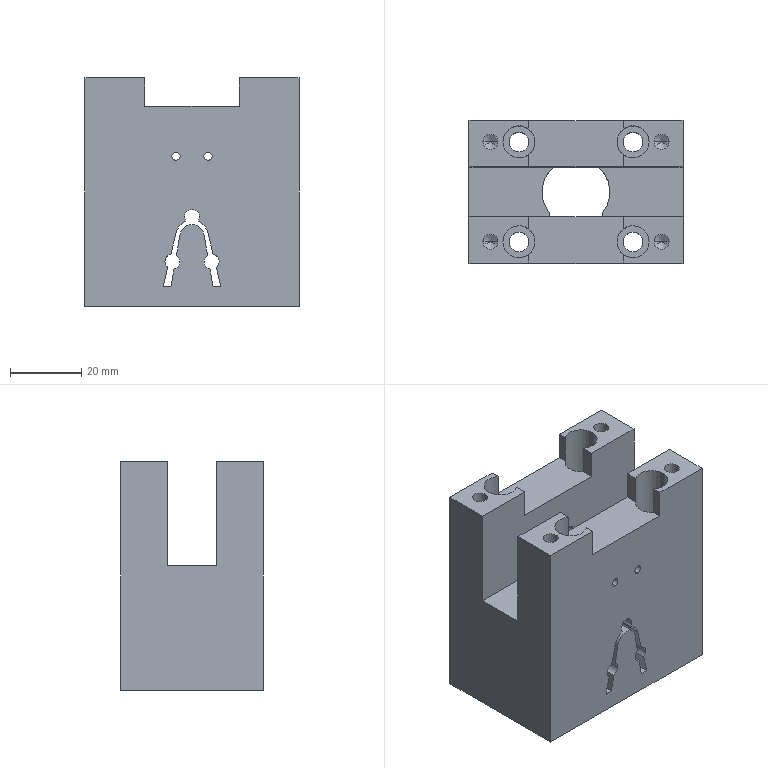Part | STEP file | magnet input block | 1 solid | 116 faces | box 60 x 40 x 64 mm | volume 101376 mm3 | plane 57 | cylinder 51 | cone 8 | commonest cylinder face diameters 4.2 x18 2.3 x8 5.5 x8 9 x8 9.2 x4 19 x3